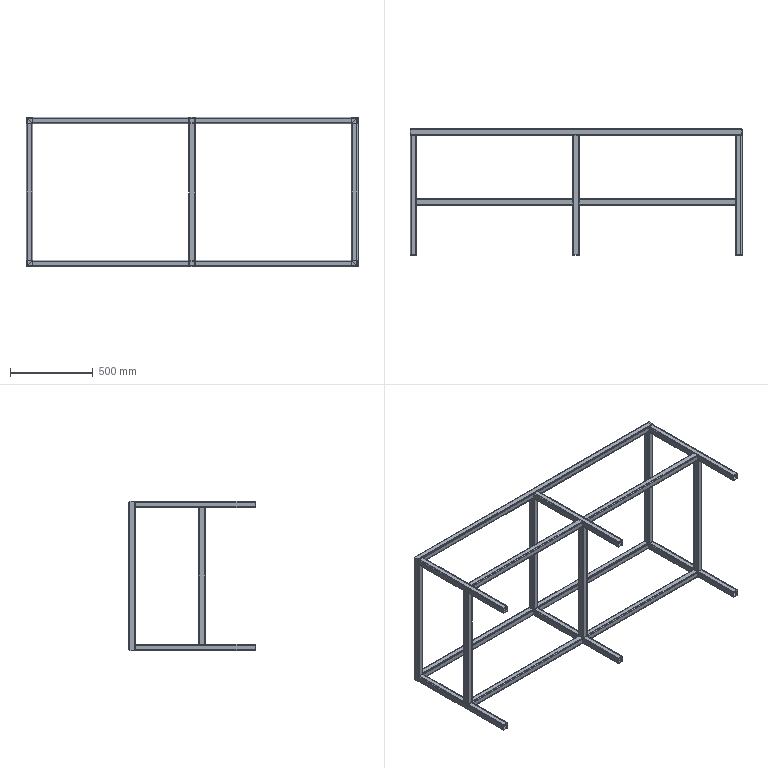Part | SolidWorks | features 3DProfileFeature 1, CosmeticWeldCutList 1, WeldMemberFeat 1, WeldmentFeature 1 | 18 solids | 324 faces | box 2000 x 760 x 900 mm | volume 7559385 mm3 | plane 180 | cylinder 144 | commonest cylinder face diameters 6.4 x72 12.8 x72